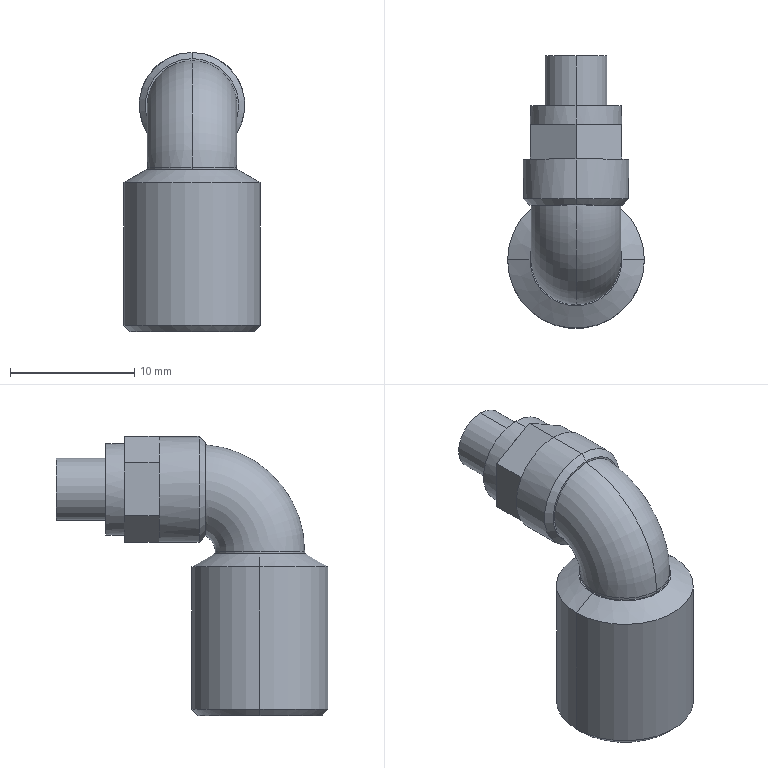Part | NX | features BREP 1 | 1 solid | 49 faces | box 11 x 21.9 x 22.45 mm | volume 1793 mm3 | plane 25 | cylinder 14 | cone 8 | torus 2 | commonest cylinder face diameters 3 x2 4 x2 5 x2 7.2 x2 7.361 x2 8.5 x2
STEP:
#1=CARTESIAN_POINT('',(0.,3.6,0.2));
#2=VERTEX_POINT('',#1);
#3=CARTESIAN_POINT('',(0.,-3.6,0.2));
#4=VERTEX_POINT('',#3);
#5=CARTESIAN_POINT('',(0.,0.,0.2));
#6=DIRECTION('',(0.,0.,1.));
#7=DIRECTION('',(1.,0.,0.));
#8=AXIS2_PLACEMENT_3D('',#5,#6,#7);
#9=CIRCLE('',#8,3.6);
#10=EDGE_CURVE('',#2,#4,#9,.T.);
#11=ORIENTED_EDGE('',*,*,#10,.T.);
#12=CARTESIAN_POINT('',(0.,4.4,8.779));
#13=VERTEX_POINT('',#12);
#14=CARTESIAN_POINT('',(0.,5.,0.2));
#15=DIRECTION('',(-1.,0.,0.));
#16=DIRECTION('',(0.,0.,1.));
#17=AXIS2_PLACEMENT_3D('',#14,#15,#16);
#18=CIRCLE('',#17,8.6);
#19=EDGE_CURVE('',#13,#4,#18,.F.);
#20=ORIENTED_EDGE('',*,*,#19,.F.);
#21=CARTESIAN_POINT('',(0.,4.4,1.465));
#22=VERTEX_POINT('',#21);
#23=CARTESIAN_POINT('',(0.,4.4,1.465));
#24=CARTESIAN_POINT('',(-0.9417,4.4,1.465));
#25=CARTESIAN_POINT('',(-2.338,4.4,2.115));
#26=CARTESIAN_POINT('',(-3.407,4.4,3.706));
#27=CARTESIAN_POINT('',(-3.681,4.4,5.191));
#28=CARTESIAN_POINT('',(-3.504,4.4,6.182));
#29=CARTESIAN_POINT('',(-3.089,4.4,7.086));
#30=CARTESIAN_POINT('',(-2.377,4.4,7.966));
#31=CARTESIAN_POINT('',(-1.516,4.4,8.531));
#32=CARTESIAN_POINT('',(-0.5014,4.4,8.779));
#33=CARTESIAN_POINT('',(0.,4.4,8.779));
#34=B_SPLINE_CURVE_WITH_KNOTS('',3,(#23,#24,#25,#26,#27,#28,#29,#30,#31,#32,#33),.UNSPECIFIED.,.F.,.F.,(4,1,1,1,1,1,1,1,4),(0.,0.25,0.375,0.5,0.625,0.6875,0.75,0.875,1.),.UNSPECIFIED.);
#35=EDGE_CURVE('',#13,#22,#34,.F.);
#36=ORIENTED_EDGE('',*,*,#35,.T.);
#37=CARTESIAN_POINT('',(0.,5.,0.2));
#38=DIRECTION('',(-1.,0.,0.));
#39=DIRECTION('',(0.,0.,1.));
#40=AXIS2_PLACEMENT_3D('',#37,#38,#39);
#41=CIRCLE('',#40,1.4);
#42=EDGE_CURVE('',#22,#2,#41,.F.);
#43=ORIENTED_EDGE('',*,*,#42,.T.);
#44=EDGE_LOOP('',(#11,#20,#36,#43));
#45=FACE_BOUND('',#44,.T.);
#46=CARTESIAN_POINT('',(0.,5.,0.2));
#47=DIRECTION('',(-1.,0.,0.));
#48=DIRECTION('',(0.,0.,1.));
#49=AXIS2_PLACEMENT_3D('',#46,#47,#48);
#50=TOROIDAL_SURFACE('',#49,5.,3.6);
#51=ADVANCED_FACE('',(#45),#50,.T.);
#52=CARTESIAN_POINT('',(0.,12.4,3.7));
#53=VERTEX_POINT('',#52);
#54=CARTESIAN_POINT('',(0.,12.4,6.7));
#55=VERTEX_POINT('',#54);
#56=CARTESIAN_POINT('',(0.,12.4,5.2));
#57=DIRECTION('',(0.,1.,0.));
#58=DIRECTION('',(0.,0.,1.));
#59=AXIS2_PLACEMENT_3D('',#56,#57,#58);
#60=CIRCLE('',#59,1.5);
#61=EDGE_CURVE('',#53,#55,#60,.T.);
#62=ORIENTED_EDGE('',*,*,#61,.F.);
#63=CARTESIAN_POINT('',(0.,16.4,3.7));
#64=VERTEX_POINT('',#63);
#65=CARTESIAN_POINT('',(0.,12.4,3.7));
#66=DIRECTION('',(0.,1.,0.));
#67=VECTOR('',#66,1000.);
#68=LINE('',#65,#67);
#69=EDGE_CURVE('',#64,#53,#68,.F.);
#70=ORIENTED_EDGE('',*,*,#69,.F.);
#71=CARTESIAN_POINT('',(0.,16.4,6.7));
#72=VERTEX_POINT('',#71);
#73=CARTESIAN_POINT('',(0.,16.4,5.2));
#74=DIRECTION('',(0.,1.,0.));
#75=DIRECTION('',(0.,0.,1.));
#76=AXIS2_PLACEMENT_3D('',#73,#74,#75);
#77=CIRCLE('',#76,1.5);
#78=EDGE_CURVE('',#64,#72,#77,.T.);
#79=ORIENTED_EDGE('',*,*,#78,.T.);
#80=CARTESIAN_POINT('',(0.,12.4,6.7));
#81=DIRECTION('',(0.,1.,0.));
#82=VECTOR('',#81,1000.);
#83=LINE('',#80,#82);
#84=EDGE_CURVE('',#72,#55,#83,.F.);
#85=ORIENTED_EDGE('',*,*,#84,.T.);
#86=EDGE_LOOP('',(#62,#70,#79,#85));
#87=FACE_BOUND('',#86,.T.);
#88=CARTESIAN_POINT('',(0.,12.4,5.2));
#89=DIRECTION('',(0.,1.,0.));
#90=DIRECTION('',(0.,0.,1.));
#91=AXIS2_PLACEMENT_3D('',#88,#89,#90);
#92=CYLINDRICAL_SURFACE('',#91,1.5);
#93=ADVANCED_FACE('',(#87),#92,.F.);
#94=CARTESIAN_POINT('',(0.,16.4,7.7));
#95=VERTEX_POINT('',#94);
#96=CARTESIAN_POINT('',(0.,16.4,2.7));
#97=VERTEX_POINT('',#96);
#98=CARTESIAN_POINT('',(0.,16.4,5.2));
#99=DIRECTION('',(0.,1.,0.));
#100=DIRECTION('',(0.,0.,1.));
#101=AXIS2_PLACEMENT_3D('',#98,#99,#100);
#102=CIRCLE('',#101,2.5);
#103=EDGE_CURVE('',#95,#97,#102,.T.);
#104=ORIENTED_EDGE('',*,*,#103,.F.);
#105=CARTESIAN_POINT('',(0.,12.4,7.7));
#106=VERTEX_POINT('',#105);
#107=CARTESIAN_POINT('',(0.,16.4,7.7));
#108=DIRECTION('',(0.,-1.,0.));
#109=VECTOR('',#108,1000.);
#110=LINE('',#107,#109);
#111=EDGE_CURVE('',#95,#106,#110,.T.);
#112=ORIENTED_EDGE('',*,*,#111,.T.);
#113=CARTESIAN_POINT('',(0.,12.4,2.7));
#114=VERTEX_POINT('',#113);
#115=CARTESIAN_POINT('',(0.,12.4,5.2));
#116=DIRECTION('',(0.,1.,0.));
#117=DIRECTION('',(0.,0.,1.));
#118=AXIS2_PLACEMENT_3D('',#115,#116,#117);
#119=CIRCLE('',#118,2.5);
#120=EDGE_CURVE('',#106,#114,#119,.T.);
#121=ORIENTED_EDGE('',*,*,#120,.T.);
#122=CARTESIAN_POINT('',(0.,16.4,2.7));
#123=DIRECTION('',(0.,-1.,0.));
#124=VECTOR('',#123,1000.);
#125=LINE('',#122,#124);
#126=EDGE_CURVE('',#97,#114,#125,.T.);
#127=ORIENTED_EDGE('',*,*,#126,.F.);
#128=EDGE_LOOP('',(#104,#112,#121,#127));
#129=FACE_BOUND('',#128,.T.);
#130=CARTESIAN_POINT('',(0.,16.4,5.2));
#131=DIRECTION('',(0.,-1.,0.));
#132=DIRECTION('',(0.,0.,-1.));
#133=AXIS2_PLACEMENT_3D('',#130,#131,#132);
#134=CYLINDRICAL_SURFACE('',#133,2.5);
#135=ADVANCED_FACE('',(#129),#134,.T.);
#136=CARTESIAN_POINT('',(0.,12.4,8.881));
#137=VERTEX_POINT('',#136);
#138=CARTESIAN_POINT('',(0.,12.4,1.519));
#139=VERTEX_POINT('',#138);
#140=CARTESIAN_POINT('',(0.,12.4,5.2));
#141=DIRECTION('',(0.,1.,0.));
#142=DIRECTION('',(0.,0.,1.));
#143=AXIS2_PLACEMENT_3D('',#140,#141,#142);
#144=CIRCLE('',#143,3.681);
#145=EDGE_CURVE('',#137,#139,#144,.T.);
#146=ORIENTED_EDGE('',*,*,#145,.F.);
#147=CARTESIAN_POINT('',(0.,10.9,8.881));
#148=VERTEX_POINT('',#147);
#149=CARTESIAN_POINT('',(0.,12.4,8.881));
#150=DIRECTION('',(0.,-1.,0.));
#151=VECTOR('',#150,1000.);
#152=LINE('',#149,#151);
#153=EDGE_CURVE('',#137,#148,#152,.T.);
#154=ORIENTED_EDGE('',*,*,#153,.T.);
#155=CARTESIAN_POINT('',(1.84,10.9,8.387));
#156=VERTEX_POINT('',#155);
#157=CARTESIAN_POINT('',(0.,10.9,5.2));
#158=DIRECTION('',(0.,1.,0.));
#159=DIRECTION('',(0.,0.,1.));
#160=AXIS2_PLACEMENT_3D('',#157,#158,#159);
#161=CIRCLE('',#160,3.681);
#162=EDGE_CURVE('',#148,#156,#161,.T.);
#163=ORIENTED_EDGE('',*,*,#162,.T.);
#164=CARTESIAN_POINT('',(3.681,10.9,5.2));
#165=VERTEX_POINT('',#164);
#166=CARTESIAN_POINT('',(0.,10.9,5.2));
#167=DIRECTION('',(0.,1.,0.));
#168=DIRECTION('',(0.,0.,1.));
#169=AXIS2_PLACEMENT_3D('',#166,#167,#168);
#170=CIRCLE('',#169,3.681);
#171=EDGE_CURVE('',#156,#165,#170,.T.);
#172=ORIENTED_EDGE('',*,*,#171,.T.);
#173=CARTESIAN_POINT('',(1.84,10.9,2.012));
#174=VERTEX_POINT('',#173);
#175=CARTESIAN_POINT('',(0.,10.9,5.2));
#176=DIRECTION('',(0.,1.,0.));
#177=DIRECTION('',(0.,0.,1.));
#178=AXIS2_PLACEMENT_3D('',#175,#176,#177);
#179=CIRCLE('',#178,3.681);
#180=EDGE_CURVE('',#165,#174,#179,.T.);
#181=ORIENTED_EDGE('',*,*,#180,.T.);
#182=CARTESIAN_POINT('',(0.,10.9,1.519));
#183=VERTEX_POINT('',#182);
#184=CARTESIAN_POINT('',(0.,10.9,5.2));
#185=DIRECTION('',(0.,1.,0.));
#186=DIRECTION('',(0.,0.,1.));
#187=AXIS2_PLACEMENT_3D('',#184,#185,#186);
#188=CIRCLE('',#187,3.681);
#189=EDGE_CURVE('',#174,#183,#188,.T.);
#190=ORIENTED_EDGE('',*,*,#189,.T.);
#191=CARTESIAN_POINT('',(0.,12.4,1.519));
#192=DIRECTION('',(0.,-1.,0.));
#193=VECTOR('',#192,1000.);
#194=LINE('',#191,#193);
#195=EDGE_CURVE('',#139,#183,#194,.T.);
#196=ORIENTED_EDGE('',*,*,#195,.F.);
#197=EDGE_LOOP('',(#146,#154,#163,#172,#181,#190,#196));
#198=FACE_BOUND('',#197,.T.);
#199=CARTESIAN_POINT('',(0.,12.4,5.2));
#200=DIRECTION('',(0.,-1.,0.));
#201=DIRECTION('',(0.,0.,-1.));
#202=AXIS2_PLACEMENT_3D('',#199,#200,#201);
#203=CYLINDRICAL_SURFACE('',#202,3.681);
#204=ADVANCED_FACE('',(#198),#203,.T.);
#205=CARTESIAN_POINT('',(0.,4.4,1.45));
#206=VERTEX_POINT('',#205);
#207=CARTESIAN_POINT('',(0.,4.4,8.95));
#208=VERTEX_POINT('',#207);
#209=CARTESIAN_POINT('',(0.,4.4,5.2));
#210=DIRECTION('',(0.,-1.,0.));
#211=DIRECTION('',(0.,0.,1.));
#212=AXIS2_PLACEMENT_3D('',#209,#210,#211);
#213=CIRCLE('',#212,3.75);
#214=EDGE_CURVE('',#206,#208,#213,.T.);
#215=ORIENTED_EDGE('',*,*,#214,.F.);
#216=CARTESIAN_POINT('',(0.,4.9,0.95));
#217=VERTEX_POINT('',#216);
#218=CARTESIAN_POINT('',(0.,4.9,0.95));
#219=DIRECTION('',(0.,0.7071,-0.7071));
#220=VECTOR('',#219,1000.);
#221=LINE('',#218,#220);
#222=EDGE_CURVE('',#217,#206,#221,.F.);
#223=ORIENTED_EDGE('',*,*,#222,.F.);
#224=CARTESIAN_POINT('',(0.,4.9,9.45));
#225=VERTEX_POINT('',#224);
#226=CARTESIAN_POINT('',(0.,4.9,5.2));
#227=DIRECTION('',(0.,1.,0.));
#228=DIRECTION('',(0.,0.,1.));
#229=AXIS2_PLACEMENT_3D('',#226,#227,#228);
#230=CIRCLE('',#229,4.25);
#231=EDGE_CURVE('',#225,#217,#230,.T.);
#232=ORIENTED_EDGE('',*,*,#231,.F.);
#233=CARTESIAN_POINT('',(0.,4.9,9.45));
#234=DIRECTION('',(0.,0.7071,0.7071));
#235=VECTOR('',#234,1000.);
#236=LINE('',#233,#235);
#237=EDGE_CURVE('',#225,#208,#236,.F.);
#238=ORIENTED_EDGE('',*,*,#237,.T.);
#239=EDGE_LOOP('',(#215,#223,#232,#238));
#240=FACE_BOUND('',#239,.T.);
#241=CARTESIAN_POINT('',(0.,4.9,5.2));
#242=DIRECTION('',(0.,1.,0.));
#243=DIRECTION('',(0.,0.,1.));
#244=AXIS2_PLACEMENT_3D('',#241,#242,#243);
#245=CONICAL_SURFACE('',#244,4.25,0.7854);
#246=ADVANCED_FACE('',(#240),#245,.T.);
#247=CARTESIAN_POINT('',(0.,8.1,9.45));
#248=VERTEX_POINT('',#247);
#249=CARTESIAN_POINT('',(3.681,8.1,7.325));
#250=VERTEX_POINT('',#249);
#251=CARTESIAN_POINT('',(0.,8.1,5.2));
#252=DIRECTION('',(0.,1.,0.));
#253=DIRECTION('',(0.,0.,1.));
#254=AXIS2_PLACEMENT_3D('',#251,#252,#253);
#255=CIRCLE('',#254,4.25);
#256=EDGE_CURVE('',#248,#250,#255,.T.);
#257=ORIENTED_EDGE('',*,*,#256,.F.);
#258=CARTESIAN_POINT('',(0.,8.1,9.45));
#259=DIRECTION('',(0.,-1.,0.));
#260=VECTOR('',#259,1000.);
#261=LINE('',#258,#260);
#262=EDGE_CURVE('',#248,#225,#261,.T.);
#263=ORIENTED_EDGE('',*,*,#262,.T.);
#264=ORIENTED_EDGE('',*,*,#231,.T.);
#265=CARTESIAN_POINT('',(0.,8.1,0.95));
#266=VERTEX_POINT('',#265);
#267=CARTESIAN_POINT('',(0.,8.1,0.95));
#268=DIRECTION('',(0.,-1.,0.));
#269=VECTOR('',#268,1000.);
#270=LINE('',#267,#269);
#271=EDGE_CURVE('',#266,#217,#270,.T.);
#272=ORIENTED_EDGE('',*,*,#271,.F.);
#273=CARTESIAN_POINT('',(3.681,8.1,3.075));
#274=VERTEX_POINT('',#273);
#275=CARTESIAN_POINT('',(0.,8.1,5.2));
#276=DIRECTION('',(0.,1.,0.));
#277=DIRECTION('',(0.,0.,1.));
#278=AXIS2_PLACEMENT_3D('',#275,#276,#277);
#279=CIRCLE('',#278,4.25);
#280=EDGE_CURVE('',#274,#266,#279,.T.);
#281=ORIENTED_EDGE('',*,*,#280,.F.);
#282=CARTESIAN_POINT('',(0.,8.1,5.2));
#283=DIRECTION('',(0.,1.,0.));
#284=DIRECTION('',(0.,0.,1.));
#285=AXIS2_PLACEMENT_3D('',#282,#283,#284);
#286=CIRCLE('',#285,4.25);
#287=EDGE_CURVE('',#250,#274,#286,.T.);
#288=ORIENTED_EDGE('',*,*,#287,.F.);
#289=EDGE_LOOP('',(#257,#263,#264,#272,#281,#288));
#290=FACE_BOUND('',#289,.T.);
#291=CARTESIAN_POINT('',(0.,8.1,5.2));
#292=DIRECTION('',(0.,-1.,0.));
#293=DIRECTION('',(0.,0.,-1.));
#294=AXIS2_PLACEMENT_3D('',#291,#292,#293);
#295=CYLINDRICAL_SURFACE('',#294,4.25);
#296=ADVANCED_FACE('',(#290),#295,.T.);
#297=CARTESIAN_POINT('',(2.,0.,-12.5));
#298=VERTEX_POINT('',#297);
#299=CARTESIAN_POINT('',(-2.,0.,-12.5));
#300=VERTEX_POINT('',#299);
#301=CARTESIAN_POINT('',(0.,0.,-12.5));
#302=DIRECTION('',(0.,0.,-1.));
#303=DIRECTION('',(-1.,0.,0.));
#304=AXIS2_PLACEMENT_3D('',#301,#302,#303);
#305=CIRCLE('',#304,2.);
#306=EDGE_CURVE('',#298,#300,#305,.T.);
#307=ORIENTED_EDGE('',*,*,#306,.F.);
#308=CARTESIAN_POINT('',(2.5,0.,-13.));
#309=VERTEX_POINT('',#308);
#310=CARTESIAN_POINT('',(2.,0.,-12.5));
#311=DIRECTION('',(0.7071,0.,-0.7071));
#312=VECTOR('',#311,1000.);
#313=LINE('',#310,#312);
#314=EDGE_CURVE('',#298,#309,#313,.T.);
#315=ORIENTED_EDGE('',*,*,#314,.T.);
#316=CARTESIAN_POINT('',(-2.5,0.,-13.));
#317=VERTEX_POINT('',#316);
#318=CARTESIAN_POINT('',(0.,0.,-13.));
#319=DIRECTION('',(0.,0.,1.));
#320=DIRECTION('',(-1.,0.,0.));
#321=AXIS2_PLACEMENT_3D('',#318,#319,#320);
#322=CIRCLE('',#321,2.5);
#323=EDGE_CURVE('',#317,#309,#322,.T.);
#324=ORIENTED_EDGE('',*,*,#323,.F.);
#325=CARTESIAN_POINT('',(-2.,0.,-12.5));
#326=DIRECTION('',(-0.7071,0.,-0.7071));
#327=VECTOR('',#326,1000.);
#328=LINE('',#325,#327);
#329=EDGE_CURVE('',#300,#317,#328,.T.);
#330=ORIENTED_EDGE('',*,*,#329,.F.);
#331=EDGE_LOOP('',(#307,#315,#324,#330));
#332=FACE_BOUND('',#331,.T.);
#333=CARTESIAN_POINT('',(0.,0.,-12.5));
#334=DIRECTION('',(0.,0.,-1.));
#335=DIRECTION('',(-1.,0.,0.));
#336=AXIS2_PLACEMENT_3D('',#333,#334,#335);
#337=CONICAL_SURFACE('',#336,2.,0.7854);
#338=ADVANCED_FACE('',(#332),#337,.F.);
#339=CARTESIAN_POINT('',(-5.,0.,-13.));
#340=VERTEX_POINT('',#339);
#341=CARTESIAN_POINT('',(5.,0.,-13.));
#342=VERTEX_POINT('',#341);
#343=CARTESIAN_POINT('',(0.,0.,-13.));
#344=DIRECTION('',(0.,0.,-1.));
#345=DIRECTION('',(-1.,0.,0.));
#346=AXIS2_PLACEMENT_3D('',#343,#344,#345);
#347=CIRCLE('',#346,5.);
#348=EDGE_CURVE('',#340,#342,#347,.T.);
#349=ORIENTED_EDGE('',*,*,#348,.F.);
#350=CARTESIAN_POINT('',(-5.5,0.,-12.5));
#351=VERTEX_POINT('',#350);
#352=CARTESIAN_POINT('',(-5.,0.,-13.));
#353=DIRECTION('',(-0.7071,0.,0.7071));
#354=VECTOR('',#353,1000.);
#355=LINE('',#352,#354);
#356=EDGE_CURVE('',#351,#340,#355,.F.);
#357=ORIENTED_EDGE('',*,*,#356,.F.);
#358=CARTESIAN_POINT('',(5.5,0.,-12.5));
#359=VERTEX_POINT('',#358);
#360=CARTESIAN_POINT('',(0.,0.,-12.5));
#361=DIRECTION('',(0.,0.,1.));
#362=DIRECTION('',(-1.,0.,0.));
#363=AXIS2_PLACEMENT_3D('',#360,#361,#362);
#364=CIRCLE('',#363,5.5);
#365=EDGE_CURVE('',#359,#351,#364,.T.);
#366=ORIENTED_EDGE('',*,*,#365,.F.);
#367=CARTESIAN_POINT('',(5.,0.,-13.));
#368=DIRECTION('',(0.7071,0.,0.7071));
#369=VECTOR('',#368,1000.);
#370=LINE('',#367,#369);
#371=EDGE_CURVE('',#359,#342,#370,.F.);
#372=ORIENTED_EDGE('',*,*,#371,.T.);
#373=EDGE_LOOP('',(#349,#357,#366,#372));
#374=FACE_BOUND('',#373,.T.);
#375=CARTESIAN_POINT('',(0.,0.,-13.));
#376=DIRECTION('',(0.,0.,1.));
#377=DIRECTION('',(1.,0.,0.));
#378=AXIS2_PLACEMENT_3D('',#375,#376,#377);
#379=CONICAL_SURFACE('',#378,5.,0.7854);
#380=ADVANCED_FACE('',(#374),#379,.T.);
#381=CARTESIAN_POINT('',(2.,0.,0.));
#382=VERTEX_POINT('',#381);
#383=CARTESIAN_POINT('',(-2.,0.,0.));
#384=VERTEX_POINT('',#383);
#385=CARTESIAN_POINT('',(0.,0.,0.));
#386=DIRECTION('',(0.,0.,-1.));
#387=DIRECTION('',(-1.,0.,0.));
#388=AXIS2_PLACEMENT_3D('',#385,#386,#387);
#389=CIRCLE('',#388,2.);
#390=EDGE_CURVE('',#382,#384,#389,.T.);
#391=ORIENTED_EDGE('',*,*,#390,.F.);
#392=CARTESIAN_POINT('',(2.,0.,0.));
#393=DIRECTION('',(0.,0.,-1.));
#394=VECTOR('',#393,1000.);
#395=LINE('',#392,#394);
#396=EDGE_CURVE('',#382,#298,#395,.T.);
#397=ORIENTED_EDGE('',*,*,#396,.T.);
#398=ORIENTED_EDGE('',*,*,#306,.T.);
#399=CARTESIAN_POINT('',(-2.,0.,0.));
#400=DIRECTION('',(0.,0.,-1.));
#401=VECTOR('',#400,1000.);
#402=LINE('',#399,#401);
#403=EDGE_CURVE('',#384,#300,#402,.T.);
#404=ORIENTED_EDGE('',*,*,#403,.F.);
#405=EDGE_LOOP('',(#391,#397,#398,#404));
#406=FACE_BOUND('',#405,.T.);
#407=CARTESIAN_POINT('',(0.,0.,0.));
#408=DIRECTION('',(0.,0.,-1.));
#409=DIRECTION('',(-1.,0.,0.));
#410=AXIS2_PLACEMENT_3D('',#407,#408,#409);
#411=CYLINDRICAL_SURFACE('',#410,2.);
#412=ADVANCED_FACE('',(#406),#411,.F.);
#413=CARTESIAN_POINT('',(3.7,0.,0.));
#414=VERTEX_POINT('',#413);
#415=CARTESIAN_POINT('',(-3.7,0.,0.));
#416=VERTEX_POINT('',#415);
#417=CARTESIAN_POINT('',(0.,0.,0.));
#418=DIRECTION('',(0.,0.,1.));
#419=DIRECTION('',(-1.,0.,0.));
#420=AXIS2_PLACEMENT_3D('',#417,#418,#419);
#421=CIRCLE('',#420,3.7);
#422=EDGE_CURVE('',#414,#416,#421,.T.);
#423=ORIENTED_EDGE('',*,*,#422,.F.);
#424=CARTESIAN_POINT('',(5.5,0.,-1.039));
#425=VERTEX_POINT('',#424);
#426=CARTESIAN_POINT('',(5.5,0.,-1.039));
#427=DIRECTION('',(0.866,0.,-0.5));
#428=VECTOR('',#427,1000.);
#429=LINE('',#426,#428);
#430=EDGE_CURVE('',#414,#425,#429,.T.);
#431=ORIENTED_EDGE('',*,*,#430,.T.);
#432=CARTESIAN_POINT('',(-5.5,0.,-1.039));
#433=VERTEX_POINT('',#432);
#434=CARTESIAN_POINT('',(0.,0.,-1.039));
#435=DIRECTION('',(0.,0.,-1.));
#436=DIRECTION('',(-1.,0.,0.));
#437=AXIS2_PLACEMENT_3D('',#434,#435,#436);
#438=CIRCLE('',#437,5.5);
#439=EDGE_CURVE('',#433,#425,#438,.T.);
#440=ORIENTED_EDGE('',*,*,#439,.F.);
#441=CARTESIAN_POINT('',(-5.5,0.,-1.039));
#442=DIRECTION('',(-0.866,0.,-0.5));
#443=VECTOR('',#442,1000.);
#444=LINE('',#441,#443);
#445=EDGE_CURVE('',#416,#433,#444,.T.);
#446=ORIENTED_EDGE('',*,*,#445,.F.);
#447=EDGE_LOOP('',(#423,#431,#440,#446));
#448=FACE_BOUND('',#447,.T.);
#449=CARTESIAN_POINT('',(0.,0.,-1.039));
#450=DIRECTION('',(0.,0.,-1.));
#451=DIRECTION('',(-1.,0.,0.));
#452=AXIS2_PLACEMENT_3D('',#449,#450,#451);
#453=CONICAL_SURFACE('',#452,5.5,1.047);
#454=ADVANCED_FACE('',(#448),#453,.T.);
#455=ORIENTED_EDGE('',*,*,#365,.T.);
#456=CARTESIAN_POINT('',(-5.5,0.,-13.));
#457=DIRECTION('',(0.,0.,1.));
#458=VECTOR('',#457,1000.);
#459=LINE('',#456,#458);
#460=EDGE_CURVE('',#433,#351,#459,.F.);
#461=ORIENTED_EDGE('',*,*,#460,.F.);
#462=ORIENTED_EDGE('',*,*,#439,.T.);
#463=CARTESIAN_POINT('',(5.5,0.,-13.));
#464=DIRECTION('',(0.,0.,1.));
#465=VECTOR('',#464,1000.);
#466=LINE('',#463,#465);
#467=EDGE_CURVE('',#425,#359,#466,.F.);
#468=ORIENTED_EDGE('',*,*,#467,.T.);
#469=EDGE_LOOP('',(#455,#461,#462,#468));
#470=FACE_BOUND('',#469,.T.);
#471=CARTESIAN_POINT('',(0.,0.,-13.));
#472=DIRECTION('',(0.,0.,1.));
#473=DIRECTION('',(1.,0.,0.));
#474=AXIS2_PLACEMENT_3D('',#471,#472,#473);
#475=CYLINDRICAL_SURFACE('',#474,5.5);
#476=ADVANCED_FACE('',(#470),#475,.T.);
#477=CARTESIAN_POINT('',(0.,0.,0.2));
#478=DIRECTION('',(0.,0.,1.));
#479=DIRECTION('',(1.,0.,0.));
#480=AXIS2_PLACEMENT_3D('',#477,#478,#479);
#481=CIRCLE('',#480,3.6);
#482=EDGE_CURVE('',#4,#2,#481,.T.);
#483=ORIENTED_EDGE('',*,*,#482,.F.);
#484=CARTESIAN_POINT('',(0.,-3.6,0.));
#485=VERTEX_POINT('',#484);
#486=CARTESIAN_POINT('',(0.,-3.6,0.2));
#487=DIRECTION('',(0.,0.,-1.));
#488=VECTOR('',#487,1000.);
#489=LINE('',#486,#488);
#490=EDGE_CURVE('',#485,#4,#489,.F.);
#491=ORIENTED_EDGE('',*,*,#490,.F.);
#492=CARTESIAN_POINT('',(0.,3.6,0.));
#493=VERTEX_POINT('',#492);
#494=CARTESIAN_POINT('',(0.,0.,0.));
#495=DIRECTION('',(0.,0.,-1.));
#496=DIRECTION('',(-1.,0.,0.));
#497=AXIS2_PLACEMENT_3D('',#494,#495,#496);
#498=CIRCLE('',#497,3.6);
#499=EDGE_CURVE('',#493,#485,#498,.T.);
#500=ORIENTED_EDGE('',*,*,#499,.F.);
#501=CARTESIAN_POINT('',(0.,3.6,0.2));
#502=DIRECTION('',(0.,0.,-1.));
#503=VECTOR('',#502,1000.);
#504=LINE('',#501,#503);
#505=EDGE_CURVE('',#493,#2,#504,.F.);
#506=ORIENTED_EDGE('',*,*,#505,.T.);
#507=EDGE_LOOP('',(#483,#491,#500,#506));
#508=FACE_BOUND('',#507,.T.);
#509=CARTESIAN_POINT('',(0.,0.,0.2));
#510=DIRECTION('',(0.,0.,-1.));
#511=DIRECTION('',(0.,1.,0.));
#512=AXIS2_PLACEMENT_3D('',#509,#510,#511);
#513=CYLINDRICAL_SURFACE('',#512,3.6);
#514=ADVANCED_FACE('',(#508),#513,.T.);
#515=CARTESIAN_POINT('',(0.,12.4,5.2));
#516=DIRECTION('',(0.,1.,0.));
#517=DIRECTION('',(0.,0.,1.));
#518=AXIS2_PLACEMENT_3D('',#515,#516,#517);
#519=CIRCLE('',#518,3.681);
#520=EDGE_CURVE('',#139,#137,#519,.T.);
#521=ORIENTED_EDGE('',*,*,#520,.T.);
#522=ORIENTED_EDGE('',*,*,#145,.T.);
#523=EDGE_LOOP('',(#521,#522));
#524=FACE_BOUND('',#523,.T.);
#525=CARTESIAN_POINT('',(0.,12.4,5.2));
#526=DIRECTION('',(0.,1.,0.));
#527=DIRECTION('',(0.,0.,1.));
#528=AXIS2_PLACEMENT_3D('',#525,#526,#527);
#529=CIRCLE('',#528,2.5);
#530=EDGE_CURVE('',#114,#106,#529,.T.);
#531=ORIENTED_EDGE('',*,*,#530,.F.);
#532=ORIENTED_EDGE('',*,*,#120,.F.);
#533=EDGE_LOOP('',(#531,#532));
#534=FACE_BOUND('',#533,.T.);
#535=CARTESIAN_POINT('',(0.,12.4,5.2));
#536=DIRECTION('',(0.,1.,0.));
#537=DIRECTION('',(0.,0.,-1.));
#538=AXIS2_PLACEMENT_3D('',#535,#536,#537);
#539=PLANE('',#538);
#540=ADVANCED_FACE('',(#524,#534),#539,.T.);
#541=ORIENTED_EDGE('',*,*,#171,.F.);
#542=CARTESIAN_POINT('',(3.681,10.9,7.325));
#543=VERTEX_POINT('',#542);
#544=CARTESIAN_POINT('',(0.,10.9,9.45));
#545=DIRECTION('',(0.866,0.,-0.5));
#546=VECTOR('',#545,1000.);
#547=LINE('',#544,#546);
#548=EDGE_CURVE('',#156,#543,#547,.T.);
#549=ORIENTED_EDGE('',*,*,#548,.T.);
#550=CARTESIAN_POINT('',(3.681,10.9,7.325));
#551=DIRECTION('',(0.,0.,-1.));
#552=VECTOR('',#551,1000.);
#553=LINE('',#550,#552);
#554=EDGE_CURVE('',#543,#165,#553,.T.);
#555=ORIENTED_EDGE('',*,*,#554,.T.);
#556=EDGE_LOOP('',(#541,#549,#555));
#557=FACE_BOUND('',#556,.T.);
#558=CARTESIAN_POINT('',(-3.681,10.9,-1.175));
#559=DIRECTION('',(0.,1.,0.));
#560=DIRECTION('',(0.,0.,-1.));
#561=AXIS2_PLACEMENT_3D('',#558,#559,#560);
#562=PLANE('',#561);
#563=ADVANCED_FACE('',(#557),#562,.T.);
#564=ORIENTED_EDGE('',*,*,#180,.F.);
#565=CARTESIAN_POINT('',(3.681,10.9,3.075));
#566=VERTEX_POINT('',#565);
#567=CARTESIAN_POINT('',(3.681,10.9,7.325));
#568=DIRECTION('',(0.,0.,-1.));
#569=VECTOR('',#568,1000.);
#570=LINE('',#567,#569);
#571=EDGE_CURVE('',#165,#566,#570,.T.);
#572=ORIENTED_EDGE('',*,*,#571,.T.);
#573=CARTESIAN_POINT('',(3.681,10.9,3.075));
#574=DIRECTION('',(-0.866,0.,-0.5));
#575=VECTOR('',#574,1000.);
#576=LINE('',#573,#575);
#577=EDGE_CURVE('',#566,#174,#576,.T.);
#578=ORIENTED_EDGE('',*,*,#577,.T.);
#579=EDGE_LOOP('',(#564,#572,#578));
#580=FACE_BOUND('',#579,.T.);
#581=CARTESIAN_POINT('',(-3.681,10.9,-1.175));
#582=DIRECTION('',(0.,1.,0.));
#583=DIRECTION('',(0.,0.,-1.));
#584=AXIS2_PLACEMENT_3D('',#581,#582,#583);
#585=PLANE('',#584);
#586=ADVANCED_FACE('',(#580),#585,.T.);
#587=ORIENTED_EDGE('',*,*,#189,.F.);
#588=CARTESIAN_POINT('',(0.,10.9,0.95));
#589=VERTEX_POINT('',#588);
#590=CARTESIAN_POINT('',(3.681,10.9,3.075));
#591=DIRECTION('',(-0.866,0.,-0.5));
#592=VECTOR('',#591,1000.);
#593=LINE('',#590,#592);
#594=EDGE_CURVE('',#174,#589,#593,.T.);
#595=ORIENTED_EDGE('',*,*,#594,.T.);
#596=CARTESIAN_POINT('',(-1.84,10.9,2.013));
#597=VERTEX_POINT('',#596);
#598=CARTESIAN_POINT('',(0.,10.9,0.95));
#599=DIRECTION('',(-0.866,0.,0.5));
#600=VECTOR('',#599,1000.);
#601=LINE('',#598,#600);
#602=EDGE_CURVE('',#589,#597,#601,.T.);
#603=ORIENTED_EDGE('',*,*,#602,.T.);
#604=CARTESIAN_POINT('',(0.,10.9,5.2));
#605=DIRECTION('',(0.,1.,0.));
#606=DIRECTION('',(0.,0.,1.));
#607=AXIS2_PLACEMENT_3D('',#604,#605,#606);
#608=CIRCLE('',#607,3.681);
#609=EDGE_CURVE('',#183,#597,#608,.T.);
#610=ORIENTED_EDGE('',*,*,#609,.F.);
#611=EDGE_LOOP('',(#587,#595,#603,#610));
#612=FACE_BOUND('',#611,.T.);
#613=CARTESIAN_POINT('',(-3.681,10.9,-1.175));
#614=DIRECTION('',(0.,1.,0.));
#615=DIRECTION('',(0.,0.,-1.));
#616=AXIS2_PLACEMENT_3D('',#613,#614,#615);
#617=PLANE('',#616);
#618=ADVANCED_FACE('',(#612),#617,.T.);
#619=CARTESIAN_POINT('',(-3.681,10.9,5.2));
#620=VERTEX_POINT('',#619);
#621=CARTESIAN_POINT('',(0.,10.9,5.2));
#622=DIRECTION('',(0.,1.,0.));
#623=DIRECTION('',(0.,0.,1.));
#624=AXIS2_PLACEMENT_3D('',#621,#622,#623);
#625=CIRCLE('',#624,3.681);
#626=EDGE_CURVE('',#597,#620,#625,.T.);
#627=ORIENTED_EDGE('',*,*,#626,.F.);
#628=CARTESIAN_POINT('',(-3.681,10.9,3.075));
#629=VERTEX_POINT('',#628);
#630=CARTESIAN_POINT('',(0.,10.9,0.95));
#631=DIRECTION('',(-0.866,0.,0.5));
#632=VECTOR('',#631,1000.);
#633=LINE('',#630,#632);
#634=EDGE_CURVE('',#597,#629,#633,.T.);
#635=ORIENTED_EDGE('',*,*,#634,.T.);
#636=CARTESIAN_POINT('',(-3.681,10.9,3.075));
#637=DIRECTION('',(0.,0.,1.));
#638=VECTOR('',#637,1000.);
#639=LINE('',#636,#638);
#640=EDGE_CURVE('',#629,#620,#639,.T.);
#641=ORIENTED_EDGE('',*,*,#640,.T.);
#642=EDGE_LOOP('',(#627,#635,#641));
#643=FACE_BOUND('',#642,.T.);
#644=CARTESIAN_POINT('',(-3.681,10.9,-1.175));
#645=DIRECTION('',(0.,1.,0.));
#646=DIRECTION('',(0.,0.,-1.));
#647=AXIS2_PLACEMENT_3D('',#644,#645,#646);
#648=PLANE('',#647);
#649=ADVANCED_FACE('',(#643),#648,.T.);
#650=CARTESIAN_POINT('',(-1.84,10.9,8.387));
#651=VERTEX_POINT('',#650);
#652=CARTESIAN_POINT('',(0.,10.9,5.2));
#653=DIRECTION('',(0.,1.,0.));
#654=DIRECTION('',(0.,0.,1.));
#655=AXIS2_PLACEMENT_3D('',#652,#653,#654);
#656=CIRCLE('',#655,3.681);
#657=EDGE_CURVE('',#620,#651,#656,.T.);
#658=ORIENTED_EDGE('',*,*,#657,.F.);
#659=CARTESIAN_POINT('',(-3.681,10.9,7.325));
#660=VERTEX_POINT('',#659);
#661=CARTESIAN_POINT('',(-3.681,10.9,3.075));
#662=DIRECTION('',(0.,0.,1.));
#663=VECTOR('',#662,1000.);
#664=LINE('',#661,#663);
#665=EDGE_CURVE('',#620,#660,#664,.T.);
#666=ORIENTED_EDGE('',*,*,#665,.T.);
#667=CARTESIAN_POINT('',(-3.681,10.9,7.325));
#668=DIRECTION('',(0.866,0.,0.5));
#669=VECTOR('',#668,1000.);
#670=LINE('',#667,#669);
#671=EDGE_CURVE('',#660,#651,#670,.T.);
#672=ORIENTED_EDGE('',*,*,#671,.T.);
#673=EDGE_LOOP('',(#658,#666,#672));
#674=FACE_BOUND('',#673,.T.);
#675=CARTESIAN_POINT('',(-3.681,10.9,-1.175));
#676=DIRECTION('',(0.,1.,0.));
#677=DIRECTION('',(0.,0.,-1.));
#678=AXIS2_PLACEMENT_3D('',#675,#676,#677);
#679=PLANE('',#678);
#680=ADVANCED_FACE('',(#674),#679,.T.);
#681=CARTESIAN_POINT('',(3.681,8.1,3.075));
#682=DIRECTION('',(-0.866,0.,-0.5));
#683=VECTOR('',#682,1000.);
#684=LINE('',#681,#683);
#685=EDGE_CURVE('',#274,#266,#684,.T.);
#686=ORIENTED_EDGE('',*,*,#685,.F.);
#687=ORIENTED_EDGE('',*,*,#280,.T.);
#688=EDGE_LOOP('',(#686,#687));
#689=FACE_BOUND('',#688,.T.);
#690=CARTESIAN_POINT('',(0.,8.1,5.2));
#691=DIRECTION('',(0.,1.,0.));
#692=DIRECTION('',(0.,0.,-1.));
#693=AXIS2_PLACEMENT_3D('',#690,#691,#692);
#694=PLANE('',#693);
#695=ADVANCED_FACE('',(#689),#694,.T.);
#696=CARTESIAN_POINT('',(3.681,8.1,7.325));
#697=DIRECTION('',(0.,0.,-1.));
#698=VECTOR('',#697,1000.);
#699=LINE('',#696,#698);
#700=EDGE_CURVE('',#250,#274,#699,.T.);
#701=ORIENTED_EDGE('',*,*,#700,.F.);
#702=ORIENTED_EDGE('',*,*,#287,.T.);
#703=EDGE_LOOP('',(#701,#702));
#704=FACE_BOUND('',#703,.T.);
#705=CARTESIAN_POINT('',(0.,8.1,5.2));
#706=DIRECTION('',(0.,1.,0.));
#707=DIRECTION('',(0.,0.,-1.));
#708=AXIS2_PLACEMENT_3D('',#705,#706,#707);
#709=PLANE('',#708);
#710=ADVANCED_FACE('',(#704),#709,.T.);
#711=CARTESIAN_POINT('',(0.,8.1,9.45));
#712=DIRECTION('',(0.866,0.,-0.5));
#713=VECTOR('',#712,1000.);
#714=LINE('',#711,#713);
#715=EDGE_CURVE('',#248,#250,#714,.T.);
#716=ORIENTED_EDGE('',*,*,#715,.F.);
#717=ORIENTED_EDGE('',*,*,#256,.T.);
#718=EDGE_LOOP('',(#716,#717));
#719=FACE_BOUND('',#718,.T.);
#720=CARTESIAN_POINT('',(0.,8.1,5.2));
#721=DIRECTION('',(0.,1.,0.));
#722=DIRECTION('',(0.,0.,-1.));
#723=AXIS2_PLACEMENT_3D('',#720,#721,#722);
#724=PLANE('',#723);
#725=ADVANCED_FACE('',(#719),#724,.T.);
#726=CARTESIAN_POINT('',(-3.681,8.1,7.325));
#727=VERTEX_POINT('',#726);
#728=CARTESIAN_POINT('',(-3.681,8.1,7.325));
#729=DIRECTION('',(0.866,0.,0.5));
#730=VECTOR('',#729,1000.);
#731=LINE('',#728,#730);
#732=EDGE_CURVE('',#727,#248,#731,.T.);
#733=ORIENTED_EDGE('',*,*,#732,.F.);
#734=CARTESIAN_POINT('',(0.,8.1,5.2));
#735=DIRECTION('',(0.,1.,0.));
#736=DIRECTION('',(0.,0.,1.));
#737=AXIS2_PLACEMENT_3D('',#734,#735,#736);
#738=CIRCLE('',#737,4.25);
#739=EDGE_CURVE('',#727,#248,#738,.T.);
#740=ORIENTED_EDGE('',*,*,#739,.T.);
#741=EDGE_LOOP('',(#733,#740));
#742=FACE_BOUND('',#741,.T.);
#743=CARTESIAN_POINT('',(0.,8.1,5.2));
#744=DIRECTION('',(0.,1.,0.));
#745=DIRECTION('',(0.,0.,-1.));
#746=AXIS2_PLACEMENT_3D('',#743,#744,#745);
#747=PLANE('',#746);
#748=ADVANCED_FACE('',(#742),#747,.T.);
#749=CARTESIAN_POINT('',(-3.681,8.1,3.075));
#750=VERTEX_POINT('',#749);
#751=CARTESIAN_POINT('',(-3.681,8.1,3.075));
#752=DIRECTION('',(0.,0.,1.));
#753=VECTOR('',#752,1000.);
#754=LINE('',#751,#753);
#755=EDGE_CURVE('',#750,#727,#754,.T.);
#756=ORIENTED_EDGE('',*,*,#755,.F.);
#757=CARTESIAN_POINT('',(0.,8.1,5.2));
#758=DIRECTION('',(0.,1.,0.));
#759=DIRECTION('',(0.,0.,1.));
#760=AXIS2_PLACEMENT_3D('',#757,#758,#759);
#761=CIRCLE('',#760,4.25);
#762=EDGE_CURVE('',#750,#727,#761,.T.);
#763=ORIENTED_EDGE('',*,*,#762,.T.);
#764=EDGE_LOOP('',(#756,#763));
#765=FACE_BOUND('',#764,.T.);
#766=CARTESIAN_POINT('',(0.,8.1,5.2));
#767=DIRECTION('',(0.,1.,0.));
#768=DIRECTION('',(0.,0.,-1.));
#769=AXIS2_PLACEMENT_3D('',#766,#767,#768);
#770=PLANE('',#769);
#771=ADVANCED_FACE('',(#765),#770,.T.);
#772=ORIENTED_EDGE('',*,*,#19,.T.);
#773=ORIENTED_EDGE('',*,*,#482,.T.);
#774=ORIENTED_EDGE('',*,*,#42,.F.);
#775=CARTESIAN_POINT('',(0.,4.4,8.779));
#776=CARTESIAN_POINT('',(0.5012,4.4,8.779));
#777=CARTESIAN_POINT('',(1.243,4.4,8.62));
#778=CARTESIAN_POINT('',(2.068,4.4,8.146));
#779=CARTESIAN_POINT('',(2.547,4.4,7.757));
#780=CARTESIAN_POINT('',(3.093,4.4,7.08));
#781=CARTESIAN_POINT('',(3.502,4.4,6.183));
#782=CARTESIAN_POINT('',(3.682,4.4,5.189));
#783=CARTESIAN_POINT('',(3.407,4.4,3.709));
#784=CARTESIAN_POINT('',(2.343,4.4,2.12));
#785=CARTESIAN_POINT('',(0.9454,4.4,1.465));
#786=CARTESIAN_POINT('',(0.,4.4,1.465));
#787=B_SPLINE_CURVE_WITH_KNOTS('',3,(#775,#776,#777,#778,#779,#780,#781,#782,#783,#784,#785,#786),.UNSPECIFIED.,.F.,.F.,(4,1,1,1,1,1,1,1,1,4),(0.,0.125,0.1875,0.25,0.3125,0.375,0.5,0.625,0.75,1.),.UNSPECIFIED.);
#788=EDGE_CURVE('',#22,#13,#787,.F.);
#789=ORIENTED_EDGE('',*,*,#788,.T.);
#790=EDGE_LOOP('',(#772,#773,#774,#789));
#791=FACE_BOUND('',#790,.T.);
#792=CARTESIAN_POINT('',(0.,5.,0.2));
#793=DIRECTION('',(-1.,0.,0.));
#794=DIRECTION('',(0.,0.,1.));
#795=AXIS2_PLACEMENT_3D('',#792,#793,#794);
#796=TOROIDAL_SURFACE('',#795,5.,3.6);
#797=ADVANCED_FACE('',(#791),#796,.T.);
#798=ORIENTED_EDGE('',*,*,#490,.T.);
#799=ORIENTED_EDGE('',*,*,#10,.F.);
#800=ORIENTED_EDGE('',*,*,#505,.F.);
#801=CARTESIAN_POINT('',(0.,0.,0.));
#802=DIRECTION('',(0.,0.,-1.));
#803=DIRECTION('',(-1.,0.,0.));
#804=AXIS2_PLACEMENT_3D('',#801,#802,#803);
#805=CIRCLE('',#804,3.6);
#806=EDGE_CURVE('',#485,#493,#805,.T.);
#807=ORIENTED_EDGE('',*,*,#806,.F.);
#808=EDGE_LOOP('',(#798,#799,#800,#807));
#809=FACE_BOUND('',#808,.T.);
#810=CARTESIAN_POINT('',(0.,0.,0.2));
#811=DIRECTION('',(0.,0.,-1.));
#812=DIRECTION('',(0.,1.,0.));
#813=AXIS2_PLACEMENT_3D('',#810,#811,#812);
#814=CYLINDRICAL_SURFACE('',#813,3.6);
#815=ADVANCED_FACE('',(#809),#814,.T.);
#816=CARTESIAN_POINT('',(0.,0.,0.));
#817=DIRECTION('',(0.,0.,1.));
#818=DIRECTION('',(-1.,0.,0.));
#819=AXIS2_PLACEMENT_3D('',#816,#817,#818);
#820=CIRCLE('',#819,3.7);
#821=EDGE_CURVE('',#416,#414,#820,.T.);
#822=ORIENTED_EDGE('',*,*,#821,.T.);
#823=ORIENTED_EDGE('',*,*,#422,.T.);
#824=EDGE_LOOP('',(#822,#823));
#825=FACE_BOUND('',#824,.T.);
#826=ORIENTED_EDGE('',*,*,#499,.T.);
#827=ORIENTED_EDGE('',*,*,#806,.T.);
#828=EDGE_LOOP('',(#826,#827));
#829=FACE_BOUND('',#828,.T.);
#830=CARTESIAN_POINT('',(0.,0.,0.));
#831=DIRECTION('',(0.,0.,-1.));
#832=DIRECTION('',(0.,-1.,0.));
#833=AXIS2_PLACEMENT_3D('',#830,#831,#832);
#834=PLANE('',#833);
#835=ADVANCED_FACE('',(#825,#829),#834,.F.);
#836=ORIENTED_EDGE('',*,*,#460,.T.);
#837=CARTESIAN_POINT('',(0.,0.,-12.5));
#838=DIRECTION('',(0.,0.,1.));
#839=DIRECTION('',(-1.,0.,0.));
#840=AXIS2_PLACEMENT_3D('',#837,#838,#839);
#841=CIRCLE('',#840,5.5);
#842=EDGE_CURVE('',#351,#359,#841,.T.);
#843=ORIENTED_EDGE('',*,*,#842,.T.);
#844=ORIENTED_EDGE('',*,*,#467,.F.);
#845=CARTESIAN_POINT('',(0.,0.,-1.039));
#846=DIRECTION('',(0.,0.,-1.));
#847=DIRECTION('',(-1.,0.,0.));
#848=AXIS2_PLACEMENT_3D('',#845,#846,#847);
#849=CIRCLE('',#848,5.5);
#850=EDGE_CURVE('',#425,#433,#849,.T.);
#851=ORIENTED_EDGE('',*,*,#850,.T.);
#852=EDGE_LOOP('',(#836,#843,#844,#851));
#853=FACE_BOUND('',#852,.T.);
#854=CARTESIAN_POINT('',(0.,0.,-13.));
#855=DIRECTION('',(0.,0.,1.));
#856=DIRECTION('',(1.,0.,0.));
#857=AXIS2_PLACEMENT_3D('',#854,#855,#856);
#858=CYLINDRICAL_SURFACE('',#857,5.5);
#859=ADVANCED_FACE('',(#853),#858,.T.);
#860=CARTESIAN_POINT('',(0.,0.,-13.));
#861=DIRECTION('',(0.,0.,-1.));
#862=DIRECTION('',(-1.,0.,0.));
#863=AXIS2_PLACEMENT_3D('',#860,#861,#862);
#864=CIRCLE('',#863,5.);
#865=EDGE_CURVE('',#342,#340,#864,.T.);
#866=ORIENTED_EDGE('',*,*,#865,.T.);
#867=ORIENTED_EDGE('',*,*,#348,.T.);
#868=EDGE_LOOP('',(#866,#867));
#869=FACE_BOUND('',#868,.T.);
#870=ORIENTED_EDGE('',*,*,#323,.T.);
#871=CARTESIAN_POINT('',(0.,0.,-13.));
#872=DIRECTION('',(0.,0.,1.));
#873=DIRECTION('',(-1.,0.,0.));
#874=AXIS2_PLACEMENT_3D('',#871,#872,#873);
#875=CIRCLE('',#874,2.5);
#876=EDGE_CURVE('',#309,#317,#875,.T.);
#877=ORIENTED_EDGE('',*,*,#876,.T.);
#878=EDGE_LOOP('',(#870,#877));
#879=FACE_BOUND('',#878,.T.);
#880=CARTESIAN_POINT('',(0.,0.,-13.));
#881=DIRECTION('',(0.,0.,-1.));
#882=DIRECTION('',(0.,-1.,0.));
#883=AXIS2_PLACEMENT_3D('',#880,#881,#882);
#884=PLANE('',#883);
#885=ADVANCED_FACE('',(#869,#879),#884,.T.);
#886=ORIENTED_EDGE('',*,*,#430,.F.);
#887=ORIENTED_EDGE('',*,*,#821,.F.);
#888=ORIENTED_EDGE('',*,*,#445,.T.);
#889=ORIENTED_EDGE('',*,*,#850,.F.);
#890=EDGE_LOOP('',(#886,#887,#888,#889));
#891=FACE_BOUND('',#890,.T.);
#892=CARTESIAN_POINT('',(0.,0.,-1.039));
#893=DIRECTION('',(0.,0.,-1.));
#894=DIRECTION('',(-1.,0.,0.));
#895=AXIS2_PLACEMENT_3D('',#892,#893,#894);
#896=CONICAL_SURFACE('',#895,5.5,1.047);
#897=ADVANCED_FACE('',(#891),#896,.T.);
#898=ORIENTED_EDGE('',*,*,#396,.F.);
#899=CARTESIAN_POINT('',(0.,0.,0.));
#900=DIRECTION('',(0.,0.,-1.));
#901=DIRECTION('',(-1.,0.,0.));
#902=AXIS2_PLACEMENT_3D('',#899,#900,#901);
#903=CIRCLE('',#902,2.);
#904=EDGE_CURVE('',#384,#382,#903,.T.);
#905=ORIENTED_EDGE('',*,*,#904,.F.);
#906=ORIENTED_EDGE('',*,*,#403,.T.);
#907=CARTESIAN_POINT('',(0.,0.,-12.5));
#908=DIRECTION('',(0.,0.,-1.));
#909=DIRECTION('',(-1.,0.,0.));
#910=AXIS2_PLACEMENT_3D('',#907,#908,#909);
#911=CIRCLE('',#910,2.);
#912=EDGE_CURVE('',#300,#298,#911,.T.);
#913=ORIENTED_EDGE('',*,*,#912,.T.);
#914=EDGE_LOOP('',(#898,#905,#906,#913));
#915=FACE_BOUND('',#914,.T.);
#916=CARTESIAN_POINT('',(0.,0.,0.));
#917=DIRECTION('',(0.,0.,-1.));
#918=DIRECTION('',(-1.,0.,0.));
#919=AXIS2_PLACEMENT_3D('',#916,#917,#918);
#920=CYLINDRICAL_SURFACE('',#919,2.);
#921=ADVANCED_FACE('',(#915),#920,.F.);
#922=ORIENTED_EDGE('',*,*,#904,.T.);
#923=ORIENTED_EDGE('',*,*,#390,.T.);
#924=EDGE_LOOP('',(#922,#923));
#925=FACE_BOUND('',#924,.T.);
#926=CARTESIAN_POINT('',(0.,0.,0.));
#927=DIRECTION('',(0.,0.,-1.));
#928=DIRECTION('',(0.,-1.,0.));
#929=AXIS2_PLACEMENT_3D('',#926,#927,#928);
#930=PLANE('',#929);
#931=ADVANCED_FACE('',(#925),#930,.T.);
#932=ORIENTED_EDGE('',*,*,#356,.T.);
#933=ORIENTED_EDGE('',*,*,#865,.F.);
#934=ORIENTED_EDGE('',*,*,#371,.F.);
#935=ORIENTED_EDGE('',*,*,#842,.F.);
#936=EDGE_LOOP('',(#932,#933,#934,#935));
#937=FACE_BOUND('',#936,.T.);
#938=CARTESIAN_POINT('',(0.,0.,-13.));
#939=DIRECTION('',(0.,0.,1.));
#940=DIRECTION('',(1.,0.,0.));
#941=AXIS2_PLACEMENT_3D('',#938,#939,#940);
#942=CONICAL_SURFACE('',#941,5.,0.7854);
#943=ADVANCED_FACE('',(#937),#942,.T.);
#944=ORIENTED_EDGE('',*,*,#314,.F.);
#945=ORIENTED_EDGE('',*,*,#912,.F.);
#946=ORIENTED_EDGE('',*,*,#329,.T.);
#947=ORIENTED_EDGE('',*,*,#876,.F.);
#948=EDGE_LOOP('',(#944,#945,#946,#947));
#949=FACE_BOUND('',#948,.T.);
#950=CARTESIAN_POINT('',(0.,0.,-12.5));
#951=DIRECTION('',(0.,0.,-1.));
#952=DIRECTION('',(-1.,0.,0.));
#953=AXIS2_PLACEMENT_3D('',#950,#951,#952);
#954=CONICAL_SURFACE('',#953,2.,0.7854);
#955=ADVANCED_FACE('',(#949),#954,.F.);
#956=CARTESIAN_POINT('',(0.,4.4,5.2));
#957=DIRECTION('',(0.,-1.,0.));
#958=DIRECTION('',(0.,0.,1.));
#959=AXIS2_PLACEMENT_3D('',#956,#957,#958);
#960=CIRCLE('',#959,3.75);
#961=EDGE_CURVE('',#208,#206,#960,.T.);
#962=ORIENTED_EDGE('',*,*,#961,.T.);
#963=ORIENTED_EDGE('',*,*,#214,.T.);
#964=EDGE_LOOP('',(#962,#963));
#965=FACE_BOUND('',#964,.T.);
#966=ORIENTED_EDGE('',*,*,#788,.F.);
#967=ORIENTED_EDGE('',*,*,#35,.F.);
#968=EDGE_LOOP('',(#966,#967));
#969=FACE_BOUND('',#968,.T.);
#970=CARTESIAN_POINT('',(0.,4.4,5.2));
#971=DIRECTION('',(0.,1.,0.));
#972=DIRECTION('',(0.,0.,-1.));
#973=AXIS2_PLACEMENT_3D('',#970,#971,#972);
#974=PLANE('',#973);
#975=ADVANCED_FACE('',(#965,#969),#974,.F.);
#976=ORIENTED_EDGE('',*,*,#262,.F.);
#977=ORIENTED_EDGE('',*,*,#739,.F.);
#978=ORIENTED_EDGE('',*,*,#762,.F.);
#979=CARTESIAN_POINT('',(0.,8.1,5.2));
#980=DIRECTION('',(0.,1.,0.));
#981=DIRECTION('',(0.,0.,1.));
#982=AXIS2_PLACEMENT_3D('',#979,#980,#981);
#983=CIRCLE('',#982,4.25);
#984=EDGE_CURVE('',#266,#750,#983,.T.);
#985=ORIENTED_EDGE('',*,*,#984,.F.);
#986=ORIENTED_EDGE('',*,*,#271,.T.);
#987=CARTESIAN_POINT('',(0.,4.9,5.2));
#988=DIRECTION('',(0.,1.,0.));
#989=DIRECTION('',(0.,0.,1.));
#990=AXIS2_PLACEMENT_3D('',#987,#988,#989);
#991=CIRCLE('',#990,4.25);
#992=EDGE_CURVE('',#217,#225,#991,.T.);
#993=ORIENTED_EDGE('',*,*,#992,.T.);
#994=EDGE_LOOP('',(#976,#977,#978,#985,#986,#993));
#995=FACE_BOUND('',#994,.T.);
#996=CARTESIAN_POINT('',(0.,8.1,5.2));
#997=DIRECTION('',(0.,-1.,0.));
#998=DIRECTION('',(0.,0.,-1.));
#999=AXIS2_PLACEMENT_3D('',#996,#997,#998);
#1000=CYLINDRICAL_SURFACE('',#999,4.25);
#1001=ADVANCED_FACE('',(#995),#1000,.T.);
#1002=CARTESIAN_POINT('',(0.,8.1,0.95));
#1003=DIRECTION('',(-0.866,0.,0.5));
#1004=VECTOR('',#1003,1000.);
#1005=LINE('',#1002,#1004);
#1006=EDGE_CURVE('',#266,#750,#1005,.T.);
#1007=ORIENTED_EDGE('',*,*,#1006,.F.);
#1008=ORIENTED_EDGE('',*,*,#984,.T.);
#1009=EDGE_LOOP('',(#1007,#1008));
#1010=FACE_BOUND('',#1009,.T.);
#1011=CARTESIAN_POINT('',(0.,8.1,5.2));
#1012=DIRECTION('',(0.,1.,0.));
#1013=DIRECTION('',(0.,0.,-1.));
#1014=AXIS2_PLACEMENT_3D('',#1011,#1012,#1013);
#1015=PLANE('',#1014);
#1016=ADVANCED_FACE('',(#1010),#1015,.T.);
#1017=ORIENTED_EDGE('',*,*,#222,.T.);
#1018=ORIENTED_EDGE('',*,*,#961,.F.);
#1019=ORIENTED_EDGE('',*,*,#237,.F.);
#1020=ORIENTED_EDGE('',*,*,#992,.F.);
#1021=EDGE_LOOP('',(#1017,#1018,#1019,#1020));
#1022=FACE_BOUND('',#1021,.T.);
#1023=CARTESIAN_POINT('',(0.,4.9,5.2));
#1024=DIRECTION('',(0.,1.,0.));
#1025=DIRECTION('',(0.,0.,1.));
#1026=AXIS2_PLACEMENT_3D('',#1023,#1024,#1025);
#1027=CONICAL_SURFACE('',#1026,4.25,0.7854);
#1028=ADVANCED_FACE('',(#1022),#1027,.T.);
#1029=ORIENTED_EDGE('',*,*,#685,.T.);
#1030=CARTESIAN_POINT('',(0.,10.9,0.95));
#1031=DIRECTION('',(0.,-1.,0.));
#1032=VECTOR('',#1031,1000.);
#1033=LINE('',#1030,#1032);
#1034=EDGE_CURVE('',#589,#266,#1033,.T.);
#1035=ORIENTED_EDGE('',*,*,#1034,.F.);
#1036=ORIENTED_EDGE('',*,*,#594,.F.);
#1037=ORIENTED_EDGE('',*,*,#577,.F.);
#1038=CARTESIAN_POINT('',(3.681,10.9,3.075));
#1039=DIRECTION('',(0.,-1.,0.));
#1040=VECTOR('',#1039,1000.);
#1041=LINE('',#1038,#1040);
#1042=EDGE_CURVE('',#566,#274,#1041,.T.);
#1043=ORIENTED_EDGE('',*,*,#1042,.T.);
#1044=EDGE_LOOP('',(#1029,#1035,#1036,#1037,#1043));
#1045=FACE_BOUND('',#1044,.T.);
#1046=CARTESIAN_POINT('',(3.681,10.9,3.075));
#1047=DIRECTION('',(-0.5,0.,0.866));
#1048=DIRECTION('',(0.,1.,0.));
#1049=AXIS2_PLACEMENT_3D('',#1046,#1047,#1048);
#1050=PLANE('',#1049);
#1051=ADVANCED_FACE('',(#1045),#1050,.F.);
#1052=ORIENTED_EDGE('',*,*,#1006,.T.);
#1053=CARTESIAN_POINT('',(-3.681,10.9,3.075));
#1054=DIRECTION('',(0.,-1.,0.));
#1055=VECTOR('',#1054,1000.);
#1056=LINE('',#1053,#1055);
#1057=EDGE_CURVE('',#629,#750,#1056,.T.);
#1058=ORIENTED_EDGE('',*,*,#1057,.F.);
#1059=ORIENTED_EDGE('',*,*,#634,.F.);
#1060=ORIENTED_EDGE('',*,*,#602,.F.);
#1061=ORIENTED_EDGE('',*,*,#1034,.T.);
#1062=EDGE_LOOP('',(#1052,#1058,#1059,#1060,#1061));
#1063=FACE_BOUND('',#1062,.T.);
#1064=CARTESIAN_POINT('',(0.,10.9,0.95));
#1065=DIRECTION('',(0.5,0.,0.866));
#1066=DIRECTION('',(0.,-1.,0.));
#1067=AXIS2_PLACEMENT_3D('',#1064,#1065,#1066);
#1068=PLANE('',#1067);
#1069=ADVANCED_FACE('',(#1063),#1068,.F.);
#1070=ORIENTED_EDGE('',*,*,#755,.T.);
#1071=CARTESIAN_POINT('',(-3.681,10.9,7.325));
#1072=DIRECTION('',(0.,-1.,0.));
#1073=VECTOR('',#1072,1000.);
#1074=LINE('',#1071,#1073);
#1075=EDGE_CURVE('',#660,#727,#1074,.T.);
#1076=ORIENTED_EDGE('',*,*,#1075,.F.);
#1077=ORIENTED_EDGE('',*,*,#665,.F.);
#1078=ORIENTED_EDGE('',*,*,#640,.F.);
#1079=ORIENTED_EDGE('',*,*,#1057,.T.);
#1080=EDGE_LOOP('',(#1070,#1076,#1077,#1078,#1079));
#1081=FACE_BOUND('',#1080,.T.);
#1082=CARTESIAN_POINT('',(-3.681,10.9,3.075));
#1083=DIRECTION('',(1.,0.,0.));
#1084=DIRECTION('',(0.,0.,-1.));
#1085=AXIS2_PLACEMENT_3D('',#1082,#1083,#1084);
#1086=PLANE('',#1085);
#1087=ADVANCED_FACE('',(#1081),#1086,.F.);
#1088=ORIENTED_EDGE('',*,*,#732,.T.);
#1089=CARTESIAN_POINT('',(0.,10.9,9.45));
#1090=VERTEX_POINT('',#1089);
#1091=CARTESIAN_POINT('',(0.,10.9,9.45));
#1092=DIRECTION('',(0.,-1.,0.));
#1093=VECTOR('',#1092,1000.);
#1094=LINE('',#1091,#1093);
#1095=EDGE_CURVE('',#1090,#248,#1094,.T.);
#1096=ORIENTED_EDGE('',*,*,#1095,.F.);
#1097=CARTESIAN_POINT('',(-3.681,10.9,7.325));
#1098=DIRECTION('',(0.866,0.,0.5));
#1099=VECTOR('',#1098,1000.);
#1100=LINE('',#1097,#1099);
#1101=EDGE_CURVE('',#651,#1090,#1100,.T.);
#1102=ORIENTED_EDGE('',*,*,#1101,.F.);
#1103=ORIENTED_EDGE('',*,*,#671,.F.);
#1104=ORIENTED_EDGE('',*,*,#1075,.T.);
#1105=EDGE_LOOP('',(#1088,#1096,#1102,#1103,#1104));
#1106=FACE_BOUND('',#1105,.T.);
#1107=CARTESIAN_POINT('',(-3.681,10.9,7.325));
#1108=DIRECTION('',(0.5,0.,-0.866));
#1109=DIRECTION('',(0.,-1.,0.));
#1110=AXIS2_PLACEMENT_3D('',#1107,#1108,#1109);
#1111=PLANE('',#1110);
#1112=ADVANCED_FACE('',(#1106),#1111,.F.);
#1113=ORIENTED_EDGE('',*,*,#715,.T.);
#1114=CARTESIAN_POINT('',(3.681,10.9,7.325));
#1115=DIRECTION('',(0.,-1.,0.));
#1116=VECTOR('',#1115,1000.);
#1117=LINE('',#1114,#1116);
#1118=EDGE_CURVE('',#543,#250,#1117,.T.);
#1119=ORIENTED_EDGE('',*,*,#1118,.F.);
#1120=ORIENTED_EDGE('',*,*,#548,.F.);
#1121=CARTESIAN_POINT('',(0.,10.9,9.45));
#1122=DIRECTION('',(0.866,0.,-0.5));
#1123=VECTOR('',#1122,1000.);
#1124=LINE('',#1121,#1123);
#1125=EDGE_CURVE('',#1090,#156,#1124,.T.);
#1126=ORIENTED_EDGE('',*,*,#1125,.F.);
#1127=ORIENTED_EDGE('',*,*,#1095,.T.);
#1128=EDGE_LOOP('',(#1113,#1119,#1120,#1126,#1127));
#1129=FACE_BOUND('',#1128,.T.);
#1130=CARTESIAN_POINT('',(0.,10.9,9.45));
#1131=DIRECTION('',(-0.5,0.,-0.866));
#1132=DIRECTION('',(-0.866,0.,0.5));
#1133=AXIS2_PLACEMENT_3D('',#1130,#1131,#1132);
#1134=PLANE('',#1133);
#1135=ADVANCED_FACE('',(#1129),#1134,.F.);
#1136=ORIENTED_EDGE('',*,*,#700,.T.);
#1137=ORIENTED_EDGE('',*,*,#1042,.F.);
#1138=ORIENTED_EDGE('',*,*,#571,.F.);
#1139=ORIENTED_EDGE('',*,*,#554,.F.);
#1140=ORIENTED_EDGE('',*,*,#1118,.T.);
#1141=EDGE_LOOP('',(#1136,#1137,#1138,#1139,#1140));
#1142=FACE_BOUND('',#1141,.T.);
#1143=CARTESIAN_POINT('',(3.681,10.9,7.325));
#1144=DIRECTION('',(-1.,0.,0.));
#1145=DIRECTION('',(0.,1.,0.));
#1146=AXIS2_PLACEMENT_3D('',#1143,#1144,#1145);
#1147=PLANE('',#1146);
#1148=ADVANCED_FACE('',(#1142),#1147,.F.);
#1149=CARTESIAN_POINT('',(0.,10.9,5.2));
#1150=DIRECTION('',(0.,1.,0.));
#1151=DIRECTION('',(0.,0.,1.));
#1152=AXIS2_PLACEMENT_3D('',#1149,#1150,#1151);
#1153=CIRCLE('',#1152,3.681);
#1154=EDGE_CURVE('',#651,#148,#1153,.T.);
#1155=ORIENTED_EDGE('',*,*,#1154,.F.);
#1156=ORIENTED_EDGE('',*,*,#1101,.T.);
#1157=ORIENTED_EDGE('',*,*,#1125,.T.);
#1158=ORIENTED_EDGE('',*,*,#162,.F.);
#1159=EDGE_LOOP('',(#1155,#1156,#1157,#1158));
#1160=FACE_BOUND('',#1159,.T.);
#1161=CARTESIAN_POINT('',(-3.681,10.9,-1.175));
#1162=DIRECTION('',(0.,1.,0.));
#1163=DIRECTION('',(0.,0.,-1.));
#1164=AXIS2_PLACEMENT_3D('',#1161,#1162,#1163);
#1165=PLANE('',#1164);
#1166=ADVANCED_FACE('',(#1160),#1165,.T.);
#1167=ORIENTED_EDGE('',*,*,#153,.F.);
#1168=ORIENTED_EDGE('',*,*,#520,.F.);
#1169=ORIENTED_EDGE('',*,*,#195,.T.);
#1170=ORIENTED_EDGE('',*,*,#609,.T.);
#1171=ORIENTED_EDGE('',*,*,#626,.T.);
#1172=ORIENTED_EDGE('',*,*,#657,.T.);
#1173=ORIENTED_EDGE('',*,*,#1154,.T.);
#1174=EDGE_LOOP('',(#1167,#1168,#1169,#1170,#1171,#1172,#1173));
#1175=FACE_BOUND('',#1174,.T.);
#1176=CARTESIAN_POINT('',(0.,12.4,5.2));
#1177=DIRECTION('',(0.,-1.,0.));
#1178=DIRECTION('',(0.,0.,-1.));
#1179=AXIS2_PLACEMENT_3D('',#1176,#1177,#1178);
#1180=CYLINDRICAL_SURFACE('',#1179,3.681);
#1181=ADVANCED_FACE('',(#1175),#1180,.T.);
#1182=ORIENTED_EDGE('',*,*,#111,.F.);
#1183=CARTESIAN_POINT('',(0.,16.4,5.2));
#1184=DIRECTION('',(0.,1.,0.));
#1185=DIRECTION('',(0.,0.,1.));
#1186=AXIS2_PLACEMENT_3D('',#1183,#1184,#1185);
#1187=CIRCLE('',#1186,2.5);
#1188=EDGE_CURVE('',#97,#95,#1187,.T.);
#1189=ORIENTED_EDGE('',*,*,#1188,.F.);
#1190=ORIENTED_EDGE('',*,*,#126,.T.);
#1191=ORIENTED_EDGE('',*,*,#530,.T.);
#1192=EDGE_LOOP('',(#1182,#1189,#1190,#1191));
#1193=FACE_BOUND('',#1192,.T.);
#1194=CARTESIAN_POINT('',(0.,16.4,5.2));
#1195=DIRECTION('',(0.,-1.,0.));
#1196=DIRECTION('',(0.,0.,-1.));
#1197=AXIS2_PLACEMENT_3D('',#1194,#1195,#1196);
#1198=CYLINDRICAL_SURFACE('',#1197,2.5);
#1199=ADVANCED_FACE('',(#1193),#1198,.T.);
#1200=ORIENTED_EDGE('',*,*,#1188,.T.);
#1201=ORIENTED_EDGE('',*,*,#103,.T.);
#1202=EDGE_LOOP('',(#1200,#1201));
#1203=FACE_BOUND('',#1202,.T.);
#1204=CARTESIAN_POINT('',(0.,16.4,5.2));
#1205=DIRECTION('',(0.,1.,0.));
#1206=DIRECTION('',(0.,0.,1.));
#1207=AXIS2_PLACEMENT_3D('',#1204,#1205,#1206);
#1208=CIRCLE('',#1207,1.5);
#1209=EDGE_CURVE('',#72,#64,#1208,.T.);
#1210=ORIENTED_EDGE('',*,*,#1209,.F.);
#1211=ORIENTED_EDGE('',*,*,#78,.F.);
#1212=EDGE_LOOP('',(#1210,#1211));
#1213=FACE_BOUND('',#1212,.T.);
#1214=CARTESIAN_POINT('',(0.,16.4,5.2));
#1215=DIRECTION('',(0.,1.,0.));
#1216=DIRECTION('',(0.,0.,-1.));
#1217=AXIS2_PLACEMENT_3D('',#1214,#1215,#1216);
#1218=PLANE('',#1217);
#1219=ADVANCED_FACE('',(#1203,#1213),#1218,.T.);
#1220=ORIENTED_EDGE('',*,*,#69,.T.);
#1221=CARTESIAN_POINT('',(0.,12.4,5.2));
#1222=DIRECTION('',(0.,1.,0.));
#1223=DIRECTION('',(0.,0.,1.));
#1224=AXIS2_PLACEMENT_3D('',#1221,#1222,#1223);
#1225=CIRCLE('',#1224,1.5);
#1226=EDGE_CURVE('',#55,#53,#1225,.T.);
#1227=ORIENTED_EDGE('',*,*,#1226,.F.);
#1228=ORIENTED_EDGE('',*,*,#84,.F.);
#1229=ORIENTED_EDGE('',*,*,#1209,.T.);
#1230=EDGE_LOOP('',(#1220,#1227,#1228,#1229));
#1231=FACE_BOUND('',#1230,.T.);
#1232=CARTESIAN_POINT('',(0.,12.4,5.2));
#1233=DIRECTION('',(0.,1.,0.));
#1234=DIRECTION('',(0.,0.,1.));
#1235=AXIS2_PLACEMENT_3D('',#1232,#1233,#1234);
#1236=CYLINDRICAL_SURFACE('',#1235,1.5);
#1237=ADVANCED_FACE('',(#1231),#1236,.F.);
#1238=ORIENTED_EDGE('',*,*,#1226,.T.);
#1239=ORIENTED_EDGE('',*,*,#61,.T.);
#1240=EDGE_LOOP('',(#1238,#1239));
#1241=FACE_BOUND('',#1240,.T.);
#1242=CARTESIAN_POINT('',(0.,12.4,5.2));
#1243=DIRECTION('',(0.,1.,0.));
#1244=DIRECTION('',(0.,0.,-1.));
#1245=AXIS2_PLACEMENT_3D('',#1242,#1243,#1244);
#1246=PLANE('',#1245);
#1247=ADVANCED_FACE('',(#1241),#1246,.T.);
#1248=CLOSED_SHELL('',(#51,#93,#135,#204,#246,#296,#338,#380,#412,#454,#476,#514,#540,#563,#586,#618,#649,#680,#695,#710,#725,#748,#771,#797,#815,#835,#859,#885,#897,#921,#931,#943,#955,#975,#1001,#1016,#1028,#1051,#1069,#1087,#1112,#1135,#1148,#1166,#1181,#1199,#1219,#1237,#1247));
#1249=MANIFOLD_SOLID_BREP('',#1248);
#1250=(LENGTH_UNIT()NAMED_UNIT(*)SI_UNIT(.MILLI.,.METRE.));
#1251=UNCERTAINTY_MEASURE_WITH_UNIT(LENGTH_MEASURE(0.0508),#1250,'','');
#1252=(NAMED_UNIT(*)PLANE_ANGLE_UNIT()SI_UNIT($,.RADIAN.));
#1253=(NAMED_UNIT(*)SI_UNIT($,.STERADIAN.)SOLID_ANGLE_UNIT());
#1254=(GEOMETRIC_REPRESENTATION_CONTEXT(3)GLOBAL_UNCERTAINTY_ASSIGNED_CONTEXT((#1251))GLOBAL_UNIT_ASSIGNED_CONTEXT((#1250,#1252,#1253))REPRESENTATION_CONTEXT('',''));
#1255=ADVANCED_BREP_SHAPE_REPRESENTATION('',(#1249),#1254);